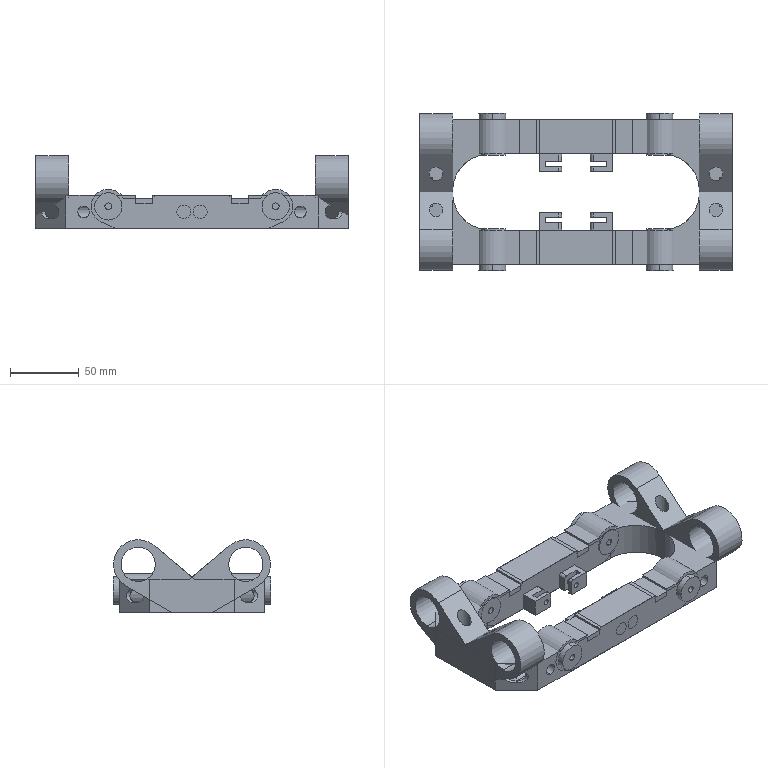NC program | Mastercam | posted with a generic post | part box 228 x 114.503 x 53 mm
Lines 5340 to 5702 of 11407:
(4 BM/BNOS |TOOL - 4|DIA. OFF. - 4|LEN. - 4|TOOL DIA. - 4.)
N856 T4 M6
N858 G0 G54 G90 X160.316 Y.34 C0. B0. S6000 M3
N860 G43 H4 Z120.
N862 Z35.841
N864 Z32.841
N866 G1 Z30.841 F600.
N868 X160.327 Y.341 Z30.552 F1500.
N870 X160.362 Y.342 Z30.265
N872 X160.418 Y.345 Z29.98
N874 X160.493 Y.348 Z29.699
N876 X160.587 Y.353 Z29.42
N878 X160.698 Y.358 Z29.146
N880 X160.825 Y.364 Z28.876
N882 X160.966 Y.371 Z28.61
N884 X161.284 Y.386 Z28.096
N886 X161.643 Y.402 Z27.607
N888 X162.03 Y.421 Z27.146
N890 X162.434 Y.44 Z26.719
N892 X162.589 Y.467 Z26.563
N894 X162.735 Y.533 Z26.414
N896 X162.872 Y.634 Z26.272
N898 X163. Y.766 Z26.139
N900 X163.118 Y.926 Z26.014
N902 X163.226 Y1.109 Z25.897
N904 X163.325 Y1.314 Z25.79
N906 X163.413 Y1.536 Z25.693
N908 X163.49 Y1.771 Z25.605
N910 X163.557 Y2.016 Z25.528
N912 X163.612 Y2.268 Z25.461
N914 X163.656 Y2.523 Z25.406
N916 X163.689 Y2.777 Z25.362
N918 X163.71 Y3.028 Z25.33
N920 X163.718 Y3.271 Z25.311
N922 X163.715 Y3.503 Z25.304
N924 X163.704 Y3.751
N926 Y4.249
N928 X163.726 Y4.745
N930 X163.769 Y5.241
N932 X163.834 Y5.734
N934 X163.921 Y6.223
N936 X164.029 Y6.709
N938 X164.158 Y7.189
N940 X164.299 Y7.634
N942 X164.459 Y8.072
N944 X164.649 Y8.532
N946 X164.858 Y8.983
N948 X165.088 Y9.424
N950 X165.336 Y9.855
N952 X165.603 Y10.274
N954 X165.888 Y10.681
N956 X166.191 Y11.076
N958 X166.511 Y11.457
N960 X166.847 Y11.823
N962 X167.199 Y12.175
N964 X167.566 Y12.51
N966 X167.947 Y12.829
N968 X168.317 Y13.114
N970 X168.699 Y13.381
N972 X169.118 Y13.649
N974 X169.549 Y13.898
N976 X169.99 Y14.128
N978 X170.44 Y14.338
N980 X170.9 Y14.529
N982 X171.367 Y14.699
N984 X171.841 Y14.848
N986 X172.321 Y14.977
N988 X172.807 Y15.084
N990 X173.297 Y15.17
N992 X173.79 Y15.235
N994 X174.285 Y15.278
N996 X174.751 Y15.299
N998 X175.218
N1000 X175.715 Y15.278
N1002 X176.21 Y15.235
N1004 X176.703 Y15.17
N1006 X177.193 Y15.084
N1008 X177.679 Y14.977
N1010 X178.159 Y14.848
N1012 X178.633 Y14.699
N1014 X179.1 Y14.529
N1016 X179.56 Y14.338
N1018 X180.01 Y14.128
N1020 X180.451 Y13.898
N1022 X180.882 Y13.649
N1024 X181.301 Y13.381
N1026 X181.683 Y13.114
N1028 X182.053 Y12.829
N1030 X182.434 Y12.51
N1032 X182.801 Y12.175
N1034 X183.153 Y11.823
N1036 X183.489 Y11.457
N1038 X183.809 Y11.076
N1040 X184.112 Y10.681
N1042 X184.397 Y10.274
N1044 X184.664 Y9.855
N1046 X184.912 Y9.424
N1048 X185.142 Y8.983
N1050 X185.351 Y8.532
N1052 X185.541 Y8.072
N1054 X185.701 Y7.634
N1056 X185.842 Y7.189
N1058 X185.971 Y6.709
N1060 X186.079 Y6.223
N1062 X186.166 Y5.734
N1064 X186.231 Y5.241
N1066 X186.274 Y4.745
N1068 X186.296 Y4.249
N1070 Y3.751
N1072 X186.274 Y3.255
N1074 X186.231 Y2.759
N1076 X186.166 Y2.266
N1078 X186.079 Y1.777
N1080 X185.971 Y1.291
N1082 X185.842 Y.811
N1084 X185.701 Y.366
N1086 X185.541 Y-.072
N1088 X185.351 Y-.532
N1090 X185.142 Y-.983
N1092 X184.912 Y-1.424
N1094 X184.664 Y-1.855
N1096 X184.397 Y-2.274
N1098 X184.112 Y-2.681
N1100 X183.809 Y-3.076
N1102 X183.489 Y-3.457
N1104 X183.153 Y-3.823
N1106 X182.801 Y-4.175
N1108 X182.434 Y-4.51
N1110 X182.053 Y-4.829
N1112 X181.683 Y-5.114
N1114 X181.301 Y-5.381
N1116 X180.882 Y-5.649
N1118 X180.451 Y-5.898
N1120 X180.01 Y-6.128
N1122 X179.56 Y-6.338
N1124 X179.1 Y-6.529
N1126 X178.633 Y-6.699
N1128 X178.159 Y-6.848
N1130 X177.679 Y-6.977
N1132 X177.193 Y-7.084
N1134 X176.703 Y-7.17
N1136 X176.21 Y-7.235
N1138 X175.715 Y-7.278
N1140 X175.249 Y-7.299
N1142 X175.031 Y-7.304
N1144 X174.782 Y-7.299
N1146 X174.285 Y-7.278
N1148 X173.79 Y-7.235
N1150 X173.297 Y-7.17
N1152 X172.807 Y-7.084
N1154 X172.321 Y-6.977
N1156 X171.841 Y-6.848
N1158 X171.367 Y-6.699
N1160 X170.9 Y-6.529
N1162 X170.44 Y-6.338
N1164 X169.99 Y-6.128
N1166 X169.549 Y-5.898
N1168 X169.118 Y-5.649
N1170 X168.699 Y-5.381
N1172 X168.317 Y-5.114
N1174 X167.947 Y-4.829
N1176 X167.566 Y-4.51
N1178 X167.199 Y-4.175
N1180 X166.847 Y-3.823
N1182 X166.511 Y-3.457
N1184 X166.191 Y-3.076
N1186 X165.888 Y-2.681
N1188 X165.603 Y-2.274
N1190 X165.336 Y-1.855
N1192 X165.088 Y-1.424
N1194 X164.858 Y-.983
N1196 X164.649 Y-.532
N1198 X164.459 Y-.072
N1200 X164.299 Y.366
N1202 X164.158 Y.811
N1204 X164.029 Y1.291
N1206 X163.921 Y1.777
N1208 X163.834 Y2.266
N1210 X163.769 Y2.759
N1212 X163.726 Y3.255
N1214 X163.715 Y3.503
N1216 X163.698 Y3.734 Z25.311
N1218 X163.668 Y3.975 Z25.33
N1220 X163.625 Y4.222 Z25.362
N1222 X163.571 Y4.473 Z25.406
N1224 X163.504 Y4.722 Z25.461
N1226 X163.427 Y4.968 Z25.528
N1228 X163.339 Y5.206 Z25.605
N1230 X163.241 Y5.433 Z25.693
N1232 X163.134 Y5.646 Z25.791
N1234 X163.018 Y5.84 Z25.898
N1236 X162.894 Y6.013 Z26.015
N1238 X162.763 Y6.161 Z26.14
N1240 X162.624 Y6.281 Z26.273
N1242 X162.479 Y6.369 Z26.414
N1244 X162.328 Y6.421 Z26.563
N1246 X162.171 Y6.434 Z26.719
N1248 X161.767 Y6.415 Z27.146
N1250 X161.38 Y6.397 Z27.607
N1252 X161.021 Y6.38 Z28.096
N1254 X160.703 Y6.365 Z28.61
N1256 X160.562 Y6.358 Z28.876
N1258 X160.435 Y6.352 Z29.146
N1260 X160.324 Y6.347 Z29.42
N1262 X160.23 Y6.343 Z29.699
N1264 X160.155 Y6.339 Z29.98
N1266 X160.099 Y6.337 Z30.265
N1268 X160.064 Y6.335 Z30.552
N1270 X160.053 Y6.334 Z30.841
N1272 G0 Z32.841
N1274 Z35.841
N1276 Z120.
N1278 X175.534 Y4.854
N1280 Z32.152
N1282 Z29.152
N1284 G1 Z27.152 F600.
N1286 X175.521 Y4.862 Z26.96 F1500.
N1288 X175.483 Y4.884 Z26.772
N1290 X175.424 Y4.919 Z26.587
N1292 X175.347 Y4.964 Z26.409
N1294 X175.256 Y5.018 Z26.237
N1296 X175.153 Y5.079 Z26.074
N1298 X174.926 Y5.213 Z25.778
N1300 X174.824 Y5.243 Z25.675
N1302 X174.706 Y5.228 Z25.583
N1304 X174.577 Y5.176 Z25.502
N1306 X174.444 Y5.094 Z25.434
N1308 X174.313 Y4.989 Z25.379
N1310 X174.188 Y4.868 Z25.339
N1312 X174.077 Y4.739 Z25.314
N1314 X173.984 Y4.609 Z25.305
N1316 X173.958 Y4.568
N1318 X173.924 Y4.497 Z25.306
N1320 X173.89 Y4.426 Z25.307
N1322 X173.872 Y4.372
N1324 X173.854 Y4.318 Z25.308
N1326 X173.841 Y4.253 Z25.307
N1328 X173.828 Y4.188 Z25.305
N1330 X173.82 Y4.108 Z25.306
N1332 X173.812 Y4.028 Z25.307
N1334 Y3.971
N1336 Y3.914 Z25.308
N1338 X173.822 Y3.85 Z25.306
N1340 X173.831 Y3.786 Z25.305
N1342 X173.854 Y3.701
N1344 X173.876 Y3.616
N1346 X173.907 Y3.54 Z25.306
N1348 X173.938 Y3.463
N1350 X173.966 Y3.413 Z25.307
N1352 X173.994 Y3.363 Z25.308
N1354 X174.031 Y3.313 Z25.306
N1356 X174.068 Y3.263 Z25.305
N1358 X174.125 Y3.201
N1360 X174.181 Y3.138 Z25.306
N1362 X174.224 Y3.1 Z25.307
N1364 X174.266 Y3.061
N1366 X174.316 Y3.027 Z25.306
N1368 X174.366 Y2.993 Z25.305
N1370 X174.444 Y2.952
N1372 X174.522 Y2.912
N1374 X174.603 Y2.882
N1376 X174.684 Y2.852
N1378 X174.741 Y2.838 Z25.306
N1380 X174.797 Y2.825 Z25.307
N1382 X174.831 Y2.821 Z25.306
N1384 X174.864 Y2.816
N1386 X174.898 Y2.812 Z25.305
N1388 X174.969 Y2.804 Z25.304
N1390 X175.072 Y2.811 Z25.305
N1392 X175.138 Y2.818 Z25.306
N1394 X175.204 Y2.825 Z25.307
N1396 X175.26 Y2.838 Z25.306
N1398 X175.316 Y2.852 Z25.305
N1400 X175.397 Y2.882
N1402 X175.478 Y2.912
N1404 X175.556 Y2.952
N1406 X175.634 Y2.993
N1408 X175.684 Y3.027 Z25.306
N1410 X175.734 Y3.061 Z25.307
N1412 X175.777 Y3.1
N1414 X175.819 Y3.138 Z25.306
N1416 X175.876 Y3.201 Z25.305
N1418 X175.932 Y3.263
N1420 X175.969 Y3.313 Z25.306
N1422 X176.006 Y3.363 Z25.308
N1424 X176.034 Y3.413 Z25.307
N1426 X176.062 Y3.463 Z25.306
N1428 X176.093 Y3.54
N1430 X176.124 Y3.616 Z25.305
N1432 X176.146 Y3.701
N1434 X176.169 Y3.786
N1436 X176.178 Y3.85 Z25.306
N1438 X176.188 Y3.914 Z25.308
N1440 Y3.971 Z25.307
N1442 Y4.028
N1444 X176.18 Y4.108 Z25.306
N1446 X176.172 Y4.188 Z25.305
N1448 X176.159 Y4.253 Z25.307
N1450 X176.146 Y4.318 Z25.308
N1452 X176.128 Y4.372 Z25.307
N1454 X176.11 Y4.426
N1456 X176.076 Y4.497 Z25.306
N1458 X176.042 Y4.568 Z25.305
N1460 X175.995 Y4.642
N1462 X175.948 Y4.716 Z25.306
N1464 X175.904 Y4.769 Z25.307
N1466 X175.861 Y4.822 Z25.308
N1468 X175.819 Y4.861 Z25.307
N1470 X175.777 Y4.899
N1472 X175.715 Y4.944 Z25.306
N1474 X175.654 Y4.99
N1476 X175.594 Y5.026 Z25.307
N1478 X175.534 Y5.062 Z25.308
N1480 X175.481 Y5.086 Z25.307
N1482 X175.429 Y5.109
N1484 X175.358 Y5.13 Z25.306
N1486 X175.286 Y5.151
N1488 X175.2 Y5.166
N1490 X175.114 Y5.182
N1492 X175.041 Y5.186 Z25.307
N1494 X174.969 Y5.19 Z25.308
N1496 X174.912 Y5.185
N1498 X174.855 Y5.18
N1500 X174.784 Y5.165 Z25.307
N1502 X174.714 Y5.151 Z25.306
N1504 X174.642 Y5.13
N1506 X174.571 Y5.109 Z25.307
N1508 X174.519 Y5.086
N1510 X174.466 Y5.062 Z25.308
N1512 X174.406 Y5.026 Z25.307
N1514 X174.346 Y4.99 Z25.306
N1516 X174.285 Y4.944
N1518 X174.223 Y4.899 Z25.307
N1520 X174.181 Y4.861
N1522 X174.139 Y4.822 Z25.308
N1524 X174.096 Y4.769 Z25.307
N1526 X174.052 Y4.716 Z25.306
N1528 X174.005 Y4.642 Z25.305
N1530 X173.984 Y4.609
N1532 X173.908 Y4.472 Z25.314
N1534 X173.84 Y4.318 Z25.34
N1536 X173.786 Y4.157 Z25.381
N1538 X173.749 Y3.995 Z25.436
N1540 X173.733 Y3.843 Z25.505
N1542 X173.742 Y3.708 Z25.585
N1544 X173.781 Y3.599 Z25.677
N1546 X173.853 Y3.525 Z25.777
N1548 X174.08 Y3.391 Z26.074
N1550 X174.183 Y3.33 Z26.237
N1552 X174.274 Y3.276 Z26.408
N1554 X174.351 Y3.231 Z26.587
N1556 X174.41 Y3.196 Z26.771
N1558 X174.448 Y3.174 Z26.96
N1560 X174.461 Y3.166 Z27.152
N1562 G0 Z29.152
N1564 Z32.152
N1566 Z120.
N1568 M5
N1570 G0 G28 G91 Z0.
N1572 G28
N1574 M01
N1576 G0 G17 G40 G80 G90 G94 G98
N1578 G0 G28 G91 Z0.